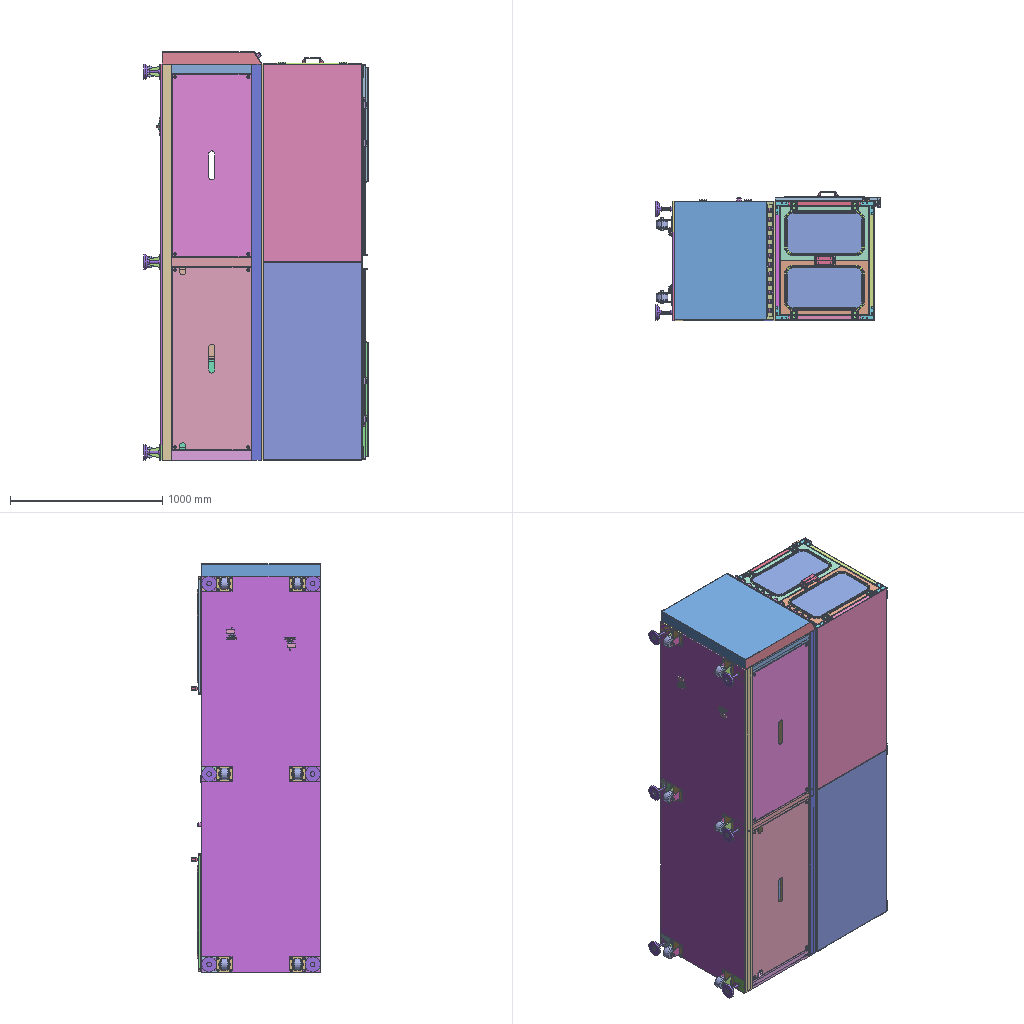Assembly | STEP file | 114 different items | 1060 placed | box 1475 x 845 x 2685 mm
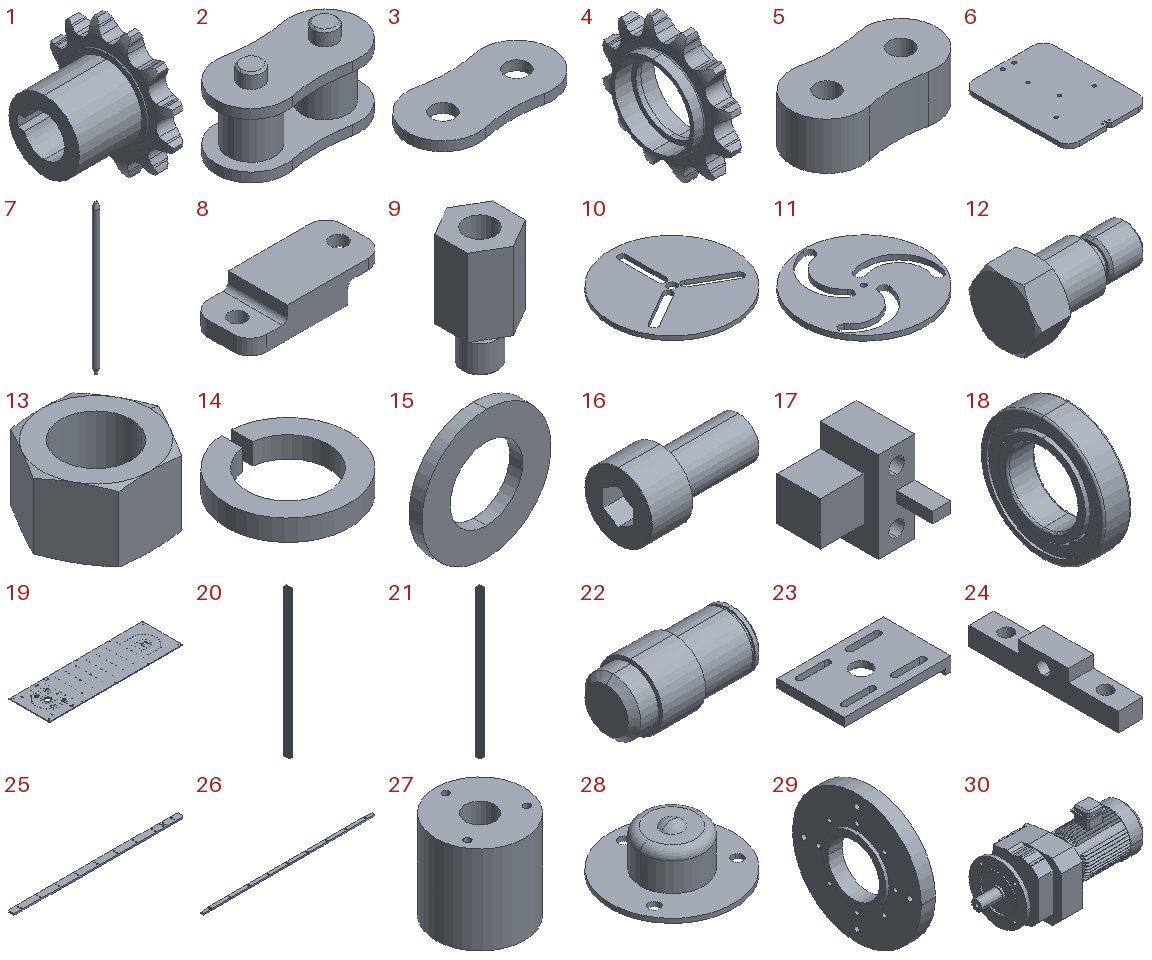Parts list (item | name | quantity | parent item | size | volume):
1 | Drive sprocket 16A-12_05B | x2 | in Chain assembly 16A (station pitch 254mm) | 70 x 105.245 x 105.245 mm | 183354 mm3
2 | Inner chain link | x80 | in Chain assembly 16A (station pitch 254mm) | 49.53 x 24.13 x 32 mm | 13899 mm3
3 | Outer chain link | x160 | in Chain assembly 16A (station pitch 254mm) | 49.79 x 24.39 x 3.25 mm | 3077 mm3
4 | Driven sprocket 16A-12_05B | x1 | in Chain assembly 16A (station pitch 254mm) | 32 x 105.245 x 105.245 mm | 65357 mm3
5 | Outer chain link pad block | x17 | in Chain assembly 16A (station pitch 254mm) | 49.79 x 24.39 x 16.175 mm | 15316 mm3
6 | Tray base | x16 | in Tooling | 180 x 235 x 10 mm | 413174 mm3
7 | Stop rod_default<machined> | x48 | in Tooling | 16 x 16 x 440 mm | 84922 mm3
8 | Guard rod seat | x48 | in Tooling | 80 x 35 x 18 mm | 32543 mm3
9 | M8X20 nut | x16 | in Tooling | 13 x 15.011 x 26.5 mm | 2477 mm3
10 | Tray plate-160 | x16 | in Tooling | 245 x 245 x 8 mm | 338994 mm3
11 | Rotary disc | x16 | in Tooling | 196 x 196 x 8 mm | 191240 mm3
12 | Tray bolt | x48 | in Tooling | 25.2 x 15.011 x 13 mm | 2145 mm3
13 | GB/T41-20001 type 1 hex nut, grade C, M8 | x48 | in Tooling | 14.2 x 12.298 x 7.9 mm | 635.641 mm3
14 | GB/T93-1987 standard spring lock washer (assembly) 8x2.1 | x48 | in Tooling | 12.277 x 12.254 x 2.1 mm | 135.755 mm3
15 | GB/T95-2002 plain washer grade C 8x1.6 | x48 | in Tooling | 16 x 1.6 x 16 mm | 219.911 mm3
16 | GB/T70.1-2000 socket head cap screw M8x16 | x16 | in Tooling | 24 x 13 x 13 mm | 1736 mm3
17 | Locating block | x16 | in Tooling | 22 x 26 x 25 mm | 4984 mm3
18 | GB/T276-94 deep groove ball bearing 6007-2Z | x2 | in Chain tooling assembly | 14 x 62 x 62 mm | 18417 mm3
19 | Silo large plate | x1 | in Silo assembly | 2600 x 780 x 12 mm | 23947596 mm3
20 | Industrial aluminium profile 3060 | x2 | in Silo assembly | 30 x 60 x 1500 mm | 776079 mm3
21 | Industrial aluminium profile 6060 | x1 | in Silo assembly | 60 x 60 x 1750 mm | 1492239 mm3
22 | Driven sprocket shaft | x1 | in Silo assembly | 79 x 40 x 40 mm | 82911 mm3
23 | Chain tension plate_default<machined> | x1 | in Silo assembly | 190 x 120 x 25 mm | 299042 mm3
24 | Driven sprocket expansion seat | x1 | in Silo assembly | 20 x 120 x 25 mm | 39515 mm3
25 | Nylon backrest plate 1 | x1 | in Silo assembly | 1900 x 69 x 16 mm | 2062797 mm3
26 | Outer nylon backrest plate 2 | x2 | in Silo assembly | 1500 x 30 x 12 mm | 516633 mm3
27 | Caster seat | x64 | in Silo assembly | 45 x 45 x 45 mm | 66141 mm3
28 | Caster wheel | x70 | in Silo assembly, Correction assembly | 45 x 45 x 17 mm | 7972 mm3
29 | Motor base plate | x1 | in Silo assembly | 27 x 200 x 200 mm | 543537 mm3
30 | NRFNRF57_NRF 27 | x1 | in Silo assembly | 502 x 221 x 222.6 mm | 8380262 mm3
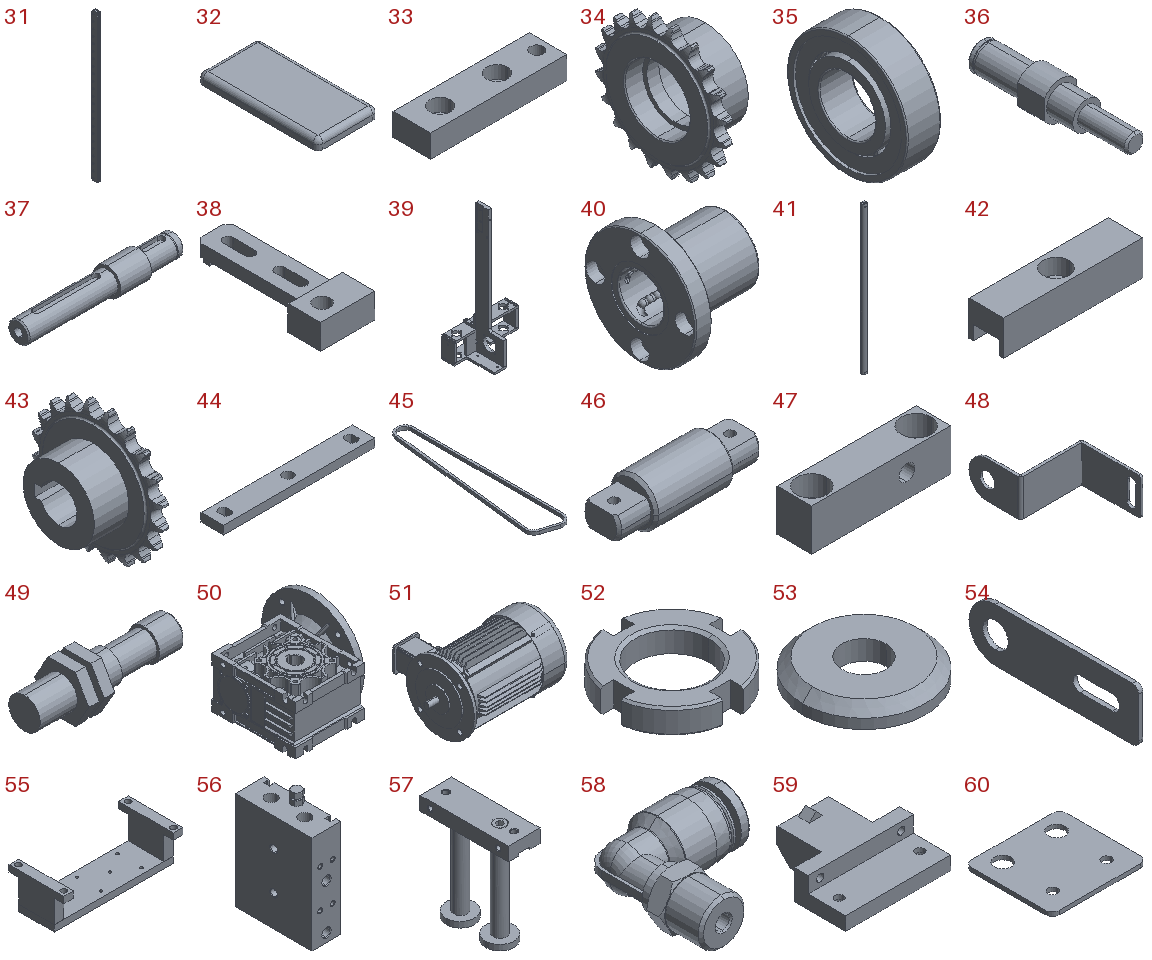31 | Flow rail_default<machined> | x4 | in Silo assembly | 46 x 62.5 x 1500 mm | 1123340 mm3
32 | Aluminium profile end cover plate | x4 | in Silo assembly | 30 x 60 x 5 mm | 8742 mm3
33 | Tensioning block | x10 | in Silo assembly | 72 x 20 x 12 mm | 15217 mm3
34 | Driven sprocket_05B | x4 | in Lifting mechanism | 24 x 64.324 x 64.324 mm | 22666 mm3
35 | Deep groove ball bearing 6002-2Z[GB/T276-94] | x8 | in Lifting mechanism | 9 x 32 x 32 mm | 3545 mm3
36 | Driven wheel shaft | x4 | in Lifting mechanism | 17 x 82.5 x 20 mm | 13654 mm3
37 | Reducer shaft | x2 | in Lifting mechanism | 131 x 23 x 23 mm | 35135 mm3
38 | Tensioner wheel bracket | x2 | in Lifting mechanism | 50 x 135 x 33 mm | 60411 mm3
39 | Lifting frame_default<machined> | x2 | in Lifting mechanism | 310 x 195 x 630 mm | 1240062 mm3
40 | LMFLMF20UU_LMF6UU | x8 | in Lifting mechanism | 42 x 54 x 54 mm | 26041 mm3
41 | Ejector rod | x4 | in Lifting mechanism | 20 x 20 x 620 mm | 192172 mm3
42 | Top plate part | x4 | in Lifting mechanism | 80 x 20 x 20 mm | 20619 mm3
43 | Drive sprocket_05B | x2 | in Lifting mechanism | 24 x 64.324 x 64.324 mm | 27131 mm3
44 | Link hanger plate | x2 | in Lifting mechanism | 270 x 40 x 15 mm | 150118 mm3
45 | Belt 1-2^Lifting mechanism | x2 | in Lifting mechanism | 133.82 x 674.32 x 12.8 mm | 154708 mm3
46 | Chain connecting rod | x2 | in Lifting mechanism | 54 x 18 x 18 mm | 10076 mm3
47 | Tensioning part | x2 | in Lifting mechanism | 60 x 15 x 18 mm | 12121 mm3
48 | Proximity switch bracket 2 | x2 | in Lifting mechanism | 52 x 90 x 30 mm | 7634 mm3
49 | Proximity switch | x6 | in Lifting mechanism, Positioning sensor assembly | 55.8 x 20.785 x 18 mm | 7139 mm3
50 | RV series aluminium alloy worm gear reducer RV40-63 | x2 | in Lifting mechanism | 120 x 160 x 140 mm | 864960 mm3
51 | Flanged end cover motor frame, no feet (TK) 63M | x2 | in Lifting mechanism | 231 x 187 x 140 mm | 1853530 mm3
52 | GB/T810-1988 small round nut M18x1.5 | x4 | in Lifting mechanism | 29.58 x 29.58 x 6 mm | 2282 mm3
53 | Small washer | x6 | in Lifting mechanism | 25 x 25 x 4 mm | 1560 mm3
54 | Proximity switch bracket 1 | x2 | in Lifting mechanism | 2 x 80 x 25 mm | 3345 mm3
55 | Cylinder mounting plate_default<machined> | x2 | in Correction assembly | 150 x 69 x 45 mm | 93928 mm3
56 | CXSM25-30(0_0)_BODY_HI | x2 | in CXSM25-30(0_0_0)_HI | 30 x 80 x 114 mm | 192548 mm3
57 | CXSM25-30(0_0)_ROD_HI | x2 | in CXSM25-30(0_0_0)_HI | 28 x 78 x 89 mm | 45235 mm3
58 | PL601_HI | x4 | in Correction assembly | 25.974 x 26.75 x 12.5 mm | 2654 mm3
59 | Correction clamp plate_default<machined> | x2 | in Correction assembly | 78 x 71 x 27 mm | 62305 mm3
60 | Sensor mounting plate | x1 | in Positioning sensor assembly | 70 x 65 x 3 mm | 12618 mm3
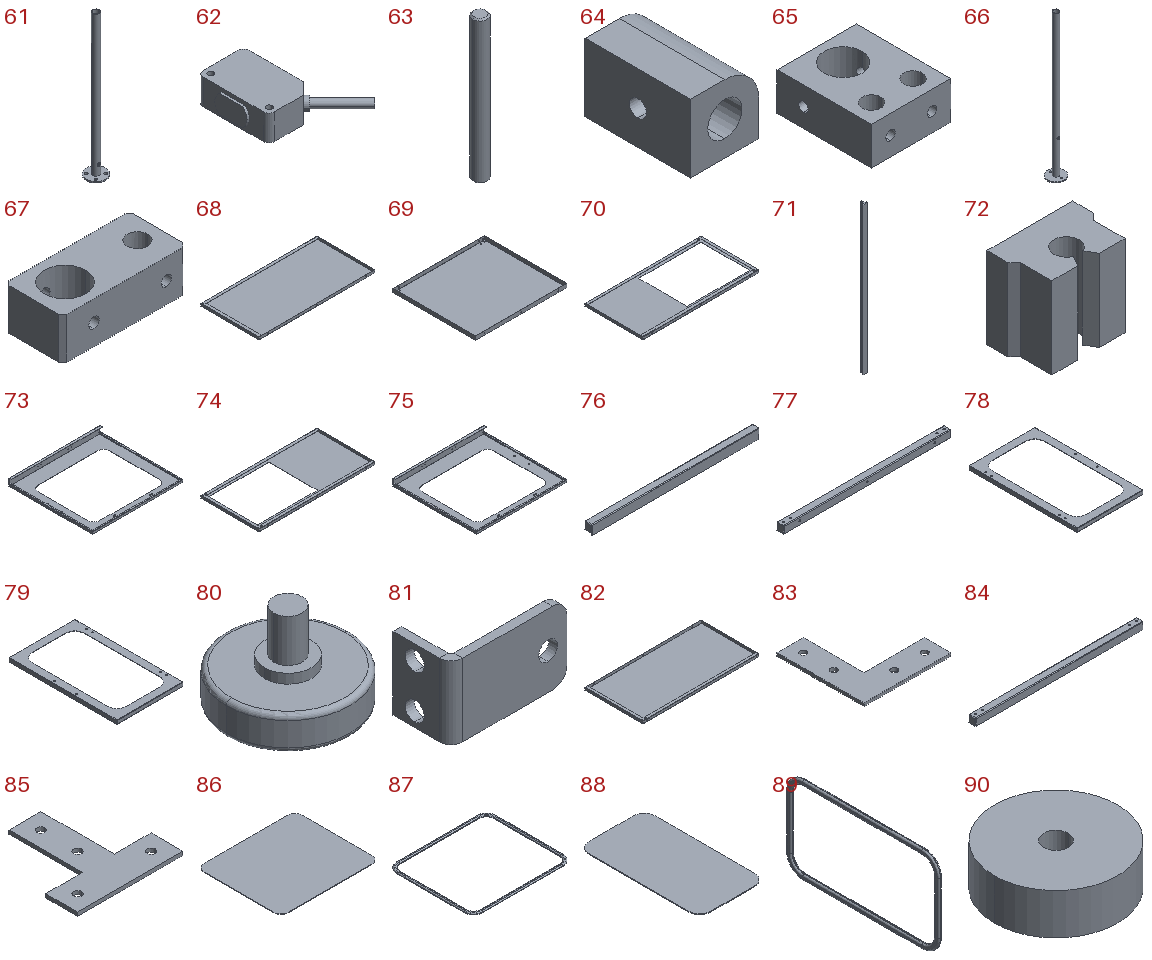61 | Switch support rod_default<machined> | x1 | in Detection mechanism | 60 x 60 x 440 mm | 47255 mm3
62 | Panasonic CX-444-P | x8 | in Detection mechanism, Sensor bracket, Sensor bracket 1 | 35.294 x 47.794 x 11.2 mm | 7023 mm3
63 | Small shaft | x8 | in Detection mechanism, Sensor bracket, Sensor bracket 1 | 10 x 10 x 100 mm | 7825 mm3
64 | Sensor mounting block | x8 | in Detection mechanism, Sensor bracket, Sensor bracket 1 | 20 x 31 x 20 mm | 9027 mm3
65 | Switch fixing block 2 | x2 | in Detection mechanism | 42 x 50 x 20 mm | 31937 mm3
66 | Switch support rod 1_default<machined> | x2 | in Sensor bracket, Sensor bracket 1 | 60 x 60 x 516 mm | 54480 mm3
67 | Switch fixing block 1 | x4 | in Sensor bracket, Sensor bracket 1 | 60 x 28 x 20 mm | 25066 mm3
68 | Inner sheet metal 1 | x1 | in Sheet metal guard | 1300 x 650 x 30 mm | 1507890 mm3
69 | Rear sheet metal | x1 | in Sheet metal guard | 720 x 650 x 30 mm | 814414 mm3
70 | Outer sheet metal | x1 | in Sheet metal guard | 1300 x 650 x 30 mm | 960013 mm3
71 | SBR16S round rail_default<machined> | x2 | in Sheet metal guard | 30 x 28.5 x 1020 mm | 387317 mm3
72 | SBR16S slide rail | x4 | in Sheet metal guard | 41 x 28 x 39 mm | 34697 mm3
73 | Sheet metal sliding door 1 | x1 | in Sheet metal guard | 750 x 690 x 61 mm | 498963 mm3
74 | Outer sheet metal 1 | x1 | in Sheet metal guard | 1300 x 650 x 30 mm | 959782 mm3
75 | Sheet metal sliding door | x1 | in Sheet metal guard | 750 x 690 x 61 mm | 498963 mm3
76 | Front sheet metal baffle | x1 | in Sheet metal guard | 720 x 30 x 40 mm | 104570 mm3
77 | Front lower sheet metal baffle | x1 | in Sheet metal guard | 720 x 30 x 30 mm | 93839 mm3
78 | Sheet metal front door | x1 | in Sheet metal guard | 360 x 588 x 21.5 mm | 195995 mm3
79 | Sheet metal front door 1 | x1 | in Sheet metal guard | 360 x 588 x 21.5 mm | 195995 mm3
80 | Nylon roller | x4 | in Sheet metal guard | 26 x 26 x 18 mm | 4094 mm3
81 | Roller hanger plate | x4 | in Sheet metal guard | 40 x 20 x 25 mm | 3864 mm3
82 | Inner sheet metal | x1 | in Sheet metal guard | 1300 x 650 x 30 mm | 1507394 mm3
83 | Outer connecting plate | x12 | in Sheet metal guard | 86 x 86 x 3 mm | 10990 mm3
84 | Middle sheet metal support plate | x1 | in Sheet metal guard | 720 x 30 x 30 mm | 93836 mm3
85 | Outer connecting plate L | x2 | in Sheet metal guard | 86 x 86 x 3 mm | 10990 mm3
86 | Glass plate | x2 | in Sheet metal guard | 580 x 500 x 3 mm | 864785 mm3
87 | Part 6^Sheet metal guard | x2 | in Sheet metal guard | 607.906 x 527.906 x 12 mm | 319171 mm3
88 | Glass plate 1 | x2 | in Sheet metal guard | 270 x 498 x 3 mm | 398165 mm3
89 | Part 8^Sheet metal guard | x2 | in Sheet metal guard | 12 x 525.906 x 297.906 mm | 225066 mm3
90 | Small locating block | x4 | in Sheet metal guard | 30 x 30 x 10 mm | 6786 mm3
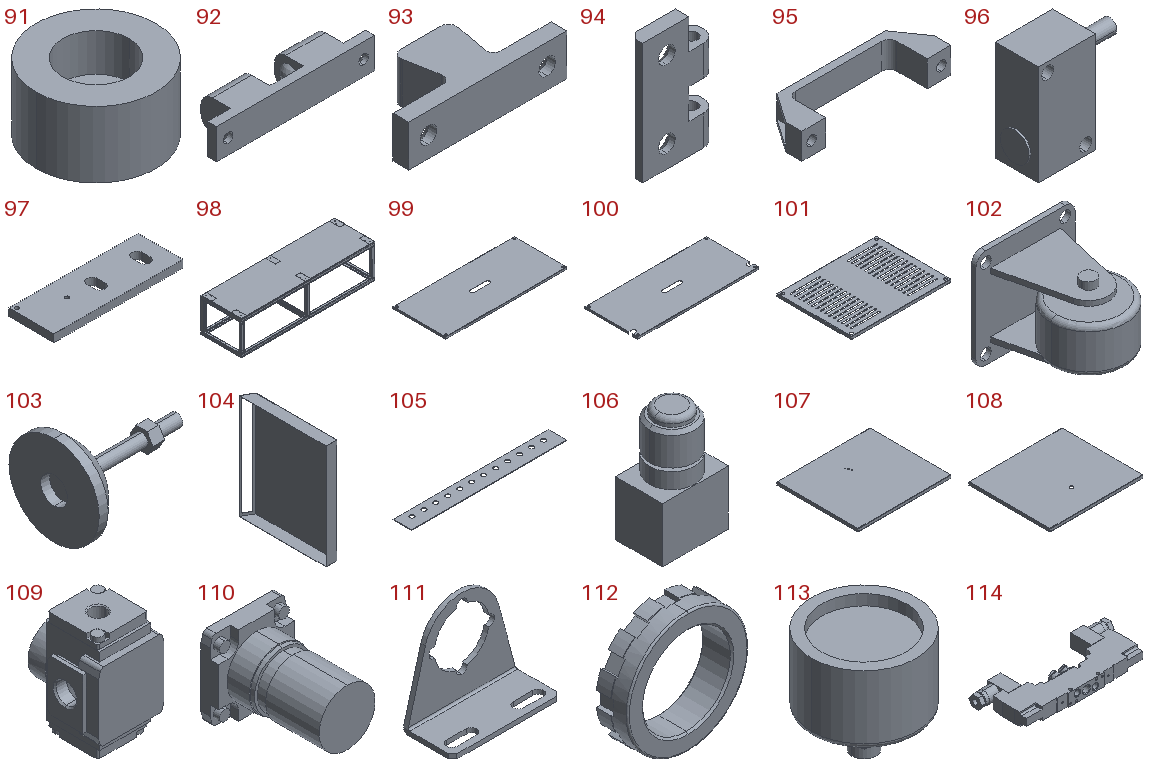91 | Buffer block | x2 | in Sheet metal guard | 18 x 18 x 10 mm | 2002 mm3
92 | Ball catch 1 | x6 | in Sheet metal guard, Box assembly | 70 x 17 x 13.5 mm | 9503 mm3
93 | Ball catch 2 | x6 | in Sheet metal guard, Box assembly | 40 x 17 x 10.5 mm | 3213 mm3
94 | Hinge CE-H3030-8-ZN | x16 | in Sheet metal guard, Box assembly | 29.8 x 10 x 49.2 mm | 6093 mm3
95 | Handle 180 | x4 | in Sheet metal guard | 138 x 42 x 24 mm | 35568 mm3
96 | Square proximity switch | x4 | in Sheet metal guard | 26.5 x 12 x 28 mm | 5309 mm3
97 | Square proximity switch plate | x2 | in Sheet metal guard | 86 x 30 x 5 mm | 12116 mm3
98 | Box 1_default<machined> | x1 | in Box assembly | 2600 x 780 x 662 mm | 45698712 mm3
99 | Box sheet metal 1_default<machined> | x2 | in Box assembly | 1203 x 522 x 20 mm | 1037743 mm3
100 | Box sheet metal 2_default<machined> | x1 | in Box assembly | 1203 x 522 x 20 mm | 1030115 mm3
101 | Box sheet metal_default<machined> | x1 | in Box assembly | 698 x 522 x 20 mm | 532626 mm3
102 | Caster_default<machined> | x6 | in Box assembly | 100 x 106 x 100 mm | 289989 mm3
103 | Foot | x6 | in Box assembly | 136 x 100 x 100 mm | 184245 mm3
104 | Push button box_default<machined> | x1 | in Box assembly | 80 x 650.121 x 780 mm | 985013 mm3
105 | Push button cover plate | x1 | in Box assembly | 780 x 92 x 3 mm | 201595 mm3
106 | Push button | x13 | in Box assembly | 42 x 30 x 72 mm | 66277 mm3
107 | Box door_default<machined> | x1 | in Box assembly | 600 x 522 x 20 mm | 571092 mm3
108 | Box door 1_default<machined> | x1 | in Box assembly | 600 x 522 x 20 mm | 570664 mm3
109 | AR20-02G(0)_BODY_HI | x1 | in AR20-02BG(0)_HI | 40 x 42.9 x 57 mm | 61556 mm3
110 | AR-20_BONNET_HI | x1 | in AR20-02BG(0)_HI | 36 x 51.1 x 37.5 mm | 33945 mm3
111 | AR20P-270AS(20)_BRACKET_HI | x1 | in AR20-02BG(0)_HI | 55 x 25.2 x 49.3 mm | 5580 mm3
112 | AR20P-260S(20)_SETNUT_HI | x1 | in AR20-02BG(0)_HI | 37.229 x 9.5 x 37.229 mm | 4541 mm3
113 | AR20-G_GAUGE_HI | x1 | in AR20-02BG(0)_HI | 37.5 x 37.5 x 37.5 mm | 25733 mm3
114 | VQZ2220-5YZ1-C6_V2_HI | x1 | in VQZ2220-5YZ1-C6_HI | 159.8 x 61.406 x 15.8 mm | 81449 mm3
Placements (level | parent | child | x y z in mm | rotation matrix by rows), first 278 of 1093 lines:
1 | subassembly 2 | Chain tooling assembly | -233.53 14.629 0.1141 | 1 0 0 0 1 0 0 0 1
2 | Chain tooling assembly | Chain assembly 16A (station pitch 254mm) | 38.756 -73.811 -756.814 | 1 0 0 0 1 0 0 0 1
3 | Chain assembly 16A (station pitch 254mm) | Drive sprocket 16A-12_05B | -13.434 74.292 1696.51 | 1 0 0 0 0.9659 -0.2588 0 0.2588 0.9659
3 | Chain assembly 16A (station pitch 254mm) | Inner chain link | -13.486 33.245 1720.208 | 0 0 -1 -0.5 -0.866 0 -0.866 0.5 0
3 | Chain assembly 16A (station pitch 254mm) | Inner chain link | -13.486 74.292 1743.907 | 0 0 -1 -1 0 0 0 1 0
3 | Chain assembly 16A (station pitch 254mm) | Inner chain link | -13.486 115.339 1720.208 | 0 0 -1 0.5 -0.866 0 -0.866 -0.5 -0
3 | Chain assembly 16A (station pitch 254mm) | Outer chain link | 0.8895 26.895 1696.51 | 0 0 -1 0 1 0 1 0 0
3 | Chain assembly 16A (station pitch 254mm) | Outer chain link | 0.8895 97.99 1737.557 | 0 0 -1 -0.866 0.5 0 0.5 0.866 0
3 | Chain assembly 16A (station pitch 254mm) | Outer chain link | 0.8895 50.593 1737.557 | 0 0 -1 -0.866 -0.5 0 -0.5 0.866 0
3 | Chain assembly 16A (station pitch 254mm) | Inner chain link | -13.486 121.689 1671.11 | 0 0 -1 0 -1 0 -1 0 -0
3 | Chain assembly 16A (station pitch 254mm) | Outer chain link | 0.8895 121.689 1696.51 | 0 0 -1 0 1 0 1 0 -0
3 | Chain assembly 16A (station pitch 254mm) | Inner chain link | -13.486 26.895 1671.11 | 0 0 -1 0 -1 0 -1 0 -0
3 | Chain assembly 16A (station pitch 254mm) | Outer chain link | 0.8895 121.689 1645.71 | 0 0 -1 0 1 0 1 0 -0
3 | Chain assembly 16A (station pitch 254mm) | Outer chain link | -24.61 121.689 1645.71 | 0 0 -1 0 1 0 1 0 -0
3 | Chain assembly 16A (station pitch 254mm) | Inner chain link | -13.486 121.689 1620.31 | 0 0 -1 0 -1 0 -1 0 -0
3 | Chain assembly 16A (station pitch 254mm) | Outer chain link | 0.8895 26.895 1645.71 | 0 0 -1 0 1 0 1 0 -0
3 | Chain assembly 16A (station pitch 254mm) | Outer chain link | -24.61 26.895 1645.71 | 0 0 -1 0 1 0 1 0 -0
3 | Chain assembly 16A (station pitch 254mm) | Inner chain link | -13.486 26.895 1620.31 | 0 0 -1 0 -1 0 -1 0 -0
3 | Chain assembly 16A (station pitch 254mm) | Outer chain link | -24.61 121.686 1594.91 | 0 0 -1 0 1 0 1 0 -0
3 | Chain assembly 16A (station pitch 254mm) | Outer chain link | -24.61 121.684 1544.11 | 0 0 -1 0 1 0 1 0 -0
3 | Chain assembly 16A (station pitch 254mm) | Outer chain link | -24.61 121.682 1493.31 | 0 0 -1 0 1 0 1 0 -0
3 | Chain assembly 16A (station pitch 254mm) | Outer chain link | -24.61 121.68 1442.51 | 0 0 -1 0 1 0 1 0 -0
3 | Chain assembly 16A (station pitch 254mm) | Outer chain link | -24.61 121.677 1391.71 | 0 0 -1 0 1 0 1 0 -0
3 | Chain assembly 16A (station pitch 254mm) | Outer chain link | -24.61 121.675 1340.91 | 0 0 -1 0 1 0 1 0 -0
3 | Chain assembly 16A (station pitch 254mm) | Outer chain link | -24.61 121.673 1290.11 | 0 0 -1 0 1 0 1 0 -0
3 | Chain assembly 16A (station pitch 254mm) | Outer chain link | -24.61 121.671 1239.31 | 0 0 -1 0 1 0 1 0 -0
3 | Chain assembly 16A (station pitch 254mm) | Outer chain link | -24.61 121.668 1188.51 | 0 0 -1 0 1 0 1 0 -0
3 | Chain assembly 16A (station pitch 254mm) | Outer chain link | -24.61 121.666 1137.71 | 0 0 -1 0 1 0 1 0 -0
3 | Chain assembly 16A (station pitch 254mm) | Outer chain link | -24.61 121.664 1086.91 | 0 0 -1 0 1 0 1 0 -0
3 | Chain assembly 16A (station pitch 254mm) | Outer chain link | -24.61 121.662 1036.11 | 0 0 -1 0 1 0 1 0 -0
3 | Chain assembly 16A (station pitch 254mm) | Outer chain link | -24.61 121.659 985.31 | 0 0 -1 0 1 0 1 0 -0
3 | Chain assembly 16A (station pitch 254mm) | Outer chain link | -24.61 121.657 934.51 | 0 0 -1 0 1 0 1 0 -0
3 | Chain assembly 16A (station pitch 254mm) | Outer chain link | -24.61 121.655 883.71 | 0 0 -1 0 1 0 1 0 -0
3 | Chain assembly 16A (station pitch 254mm) | Outer chain link | -24.61 121.653 832.91 | 0 0 -1 0 1 0 1 0 -0
3 | Chain assembly 16A (station pitch 254mm) | Outer chain link | -24.61 121.65 782.11 | 0 0 -1 0 1 0 1 0 -0
3 | Chain assembly 16A (station pitch 254mm) | Outer chain link | -24.61 121.648 731.31 | 0 0 -1 0 1 0 1 0 -0
3 | Chain assembly 16A (station pitch 254mm) | Outer chain link | -24.61 121.646 680.51 | 0 0 -1 0 1 0 1 0 -0
3 | Chain assembly 16A (station pitch 254mm) | Outer chain link | -24.61 121.644 629.71 | 0 0 -1 0 1 0 1 0 -0
3 | Chain assembly 16A (station pitch 254mm) | Outer chain link | -24.61 121.641 578.91 | 0 0 -1 0 1 0 1 0 -0
3 | Chain assembly 16A (station pitch 254mm) | Outer chain link | -24.61 121.639 528.11 | 0 0 -1 0 1 0 1 0 -0
3 | Chain assembly 16A (station pitch 254mm) | Outer chain link | -24.61 121.637 477.31 | 0 0 -1 0 1 0 1 0 -0
3 | Chain assembly 16A (station pitch 254mm) | Outer chain link | -24.61 121.634 426.51 | 0 0 -1 0 1 0 1 0 -0
3 | Chain assembly 16A (station pitch 254mm) | Outer chain link | -24.61 121.632 375.71 | 0 0 -1 0 1 0 1 0 -0
3 | Chain assembly 16A (station pitch 254mm) | Outer chain link | -24.61 121.63 324.91 | 0 0 -1 0 1 0 1 0 -0
3 | Chain assembly 16A (station pitch 254mm) | Outer chain link | -24.61 121.628 274.11 | 0 0 -1 0 1 0 1 0 -0
3 | Chain assembly 16A (station pitch 254mm) | Outer chain link | -24.61 121.625 223.31 | 0 0 -1 0 1 0 1 0 -0
3 | Chain assembly 16A (station pitch 254mm) | Outer chain link | -24.61 121.623 172.51 | 0 0 -1 0 1 0 1 0 -0
3 | Chain assembly 16A (station pitch 254mm) | Outer chain link | -24.61 121.621 121.71 | 0 0 -1 0 1 0 1 0 -0
3 | Chain assembly 16A (station pitch 254mm) | Outer chain link | -24.61 121.619 70.91 | 0 0 -1 0 1 0 1 0 -0
3 | Chain assembly 16A (station pitch 254mm) | Outer chain link | -24.61 121.616 20.11 | 0 0 -1 0 1 0 1 0 -0
3 | Chain assembly 16A (station pitch 254mm) | Outer chain link | -24.61 121.614 -30.69 | 0 0 -1 0 1 0 1 0 -0
3 | Chain assembly 16A (station pitch 254mm) | Outer chain link | -24.61 121.612 -81.49 | 0 0 -1 0 1 0 1 0 -0
3 | Chain assembly 16A (station pitch 254mm) | Outer chain link | -24.61 121.609 -132.29 | 0 0 -1 0 1 0 1 0 -0
3 | Chain assembly 16A (station pitch 254mm) | Outer chain link | 0.8895 121.686 1594.91 | 0 0 -1 0 1 0 1 0 -0
3 | Chain assembly 16A (station pitch 254mm) | Outer chain link | 0.8895 121.684 1544.11 | 0 0 -1 0 1 0 1 0 -0
3 | Chain assembly 16A (station pitch 254mm) | Outer chain link | 0.8895 121.682 1493.31 | 0 0 -1 0 1 0 1 0 -0
3 | Chain assembly 16A (station pitch 254mm) | Outer chain link | 0.8895 121.68 1442.51 | 0 0 -1 0 1 0 1 0 -0
3 | Chain assembly 16A (station pitch 254mm) | Outer chain link | 0.8895 121.677 1391.71 | 0 0 -1 0 1 0 1 0 -0
3 | Chain assembly 16A (station pitch 254mm) | Outer chain link | 0.8895 121.675 1340.91 | 0 0 -1 0 1 0 1 0 -0
3 | Chain assembly 16A (station pitch 254mm) | Outer chain link | 0.8895 121.673 1290.11 | 0 0 -1 0 1 0 1 0 -0
3 | Chain assembly 16A (station pitch 254mm) | Outer chain link | 0.8895 121.671 1239.31 | 0 0 -1 0 1 0 1 0 -0
3 | Chain assembly 16A (station pitch 254mm) | Outer chain link | 0.8895 121.668 1188.51 | 0 0 -1 0 1 0 1 0 -0
3 | Chain assembly 16A (station pitch 254mm) | Outer chain link | 0.8895 121.666 1137.71 | 0 0 -1 0 1 0 1 0 -0
3 | Chain assembly 16A (station pitch 254mm) | Outer chain link | 0.8895 121.664 1086.91 | 0 0 -1 0 1 0 1 0 -0
3 | Chain assembly 16A (station pitch 254mm) | Outer chain link | 0.8895 121.662 1036.11 | 0 0 -1 0 1 0 1 0 -0
3 | Chain assembly 16A (station pitch 254mm) | Outer chain link | 0.8895 121.659 985.31 | 0 0 -1 0 1 0 1 0 -0
3 | Chain assembly 16A (station pitch 254mm) | Outer chain link | 0.8895 121.657 934.51 | 0 0 -1 0 1 0 1 0 -0
3 | Chain assembly 16A (station pitch 254mm) | Outer chain link | 0.8895 121.655 883.71 | 0 0 -1 0 1 0 1 0 -0
3 | Chain assembly 16A (station pitch 254mm) | Outer chain link | 0.8895 121.653 832.91 | 0 0 -1 0 1 0 1 0 -0
3 | Chain assembly 16A (station pitch 254mm) | Outer chain link | 0.8895 121.65 782.11 | 0 0 -1 0 1 0 1 0 -0
3 | Chain assembly 16A (station pitch 254mm) | Outer chain link | 0.8895 121.648 731.31 | 0 0 -1 0 1 0 1 0 -0
3 | Chain assembly 16A (station pitch 254mm) | Outer chain link | 0.8895 121.646 680.51 | 0 0 -1 0 1 0 1 0 -0
3 | Chain assembly 16A (station pitch 254mm) | Outer chain link | 0.8895 121.644 629.71 | 0 0 -1 0 1 0 1 0 -0
3 | Chain assembly 16A (station pitch 254mm) | Outer chain link | 0.8895 121.641 578.91 | 0 0 -1 0 1 0 1 0 -0
3 | Chain assembly 16A (station pitch 254mm) | Outer chain link | 0.8895 121.639 528.11 | 0 0 -1 0 1 0 1 0 -0
3 | Chain assembly 16A (station pitch 254mm) | Outer chain link | 0.8895 121.637 477.31 | 0 0 -1 0 1 0 1 0 -0
3 | Chain assembly 16A (station pitch 254mm) | Outer chain link | 0.8895 121.634 426.51 | 0 0 -1 0 1 0 1 0 -0
3 | Chain assembly 16A (station pitch 254mm) | Outer chain link | 0.8895 121.632 375.71 | 0 0 -1 0 1 0 1 0 -0
3 | Chain assembly 16A (station pitch 254mm) | Outer chain link | 0.8895 121.63 324.91 | 0 0 -1 0 1 0 1 0 -0
3 | Chain assembly 16A (station pitch 254mm) | Outer chain link | 0.8895 121.628 274.11 | 0 0 -1 0 1 0 1 0 -0
3 | Chain assembly 16A (station pitch 254mm) | Outer chain link | 0.8895 121.625 223.31 | 0 0 -1 0 1 0 1 0 -0
3 | Chain assembly 16A (station pitch 254mm) | Outer chain link | 0.8895 121.623 172.51 | 0 0 -1 0 1 0 1 0 -0
3 | Chain assembly 16A (station pitch 254mm) | Outer chain link | 0.8895 121.621 121.71 | 0 0 -1 0 1 0 1 0 -0
3 | Chain assembly 16A (station pitch 254mm) | Outer chain link | 0.8895 121.619 70.91 | 0 0 -1 0 1 0 1 0 -0
3 | Chain assembly 16A (station pitch 254mm) | Outer chain link | 0.8895 121.616 20.11 | 0 0 -1 0 1 0 1 0 -0
3 | Chain assembly 16A (station pitch 254mm) | Outer chain link | 0.8895 121.614 -30.69 | 0 0 -1 0 1 0 1 0 -0
3 | Chain assembly 16A (station pitch 254mm) | Outer chain link | 0.8895 121.612 -81.49 | 0 0 -1 0 1 0 1 0 -0
3 | Chain assembly 16A (station pitch 254mm) | Outer chain link | 1.25 121.609 -132.29 | 0 0 -1 0 1 0 1 0 -0
3 | Chain assembly 16A (station pitch 254mm) | Inner chain link | -13.486 121.686 1569.51 | 0 0 -1 0 -1 0 -1 0 -0
3 | Chain assembly 16A (station pitch 254mm) | Inner chain link | -13.486 121.684 1518.71 | 0 0 -1 0 -1 0 -1 0 -0
3 | Chain assembly 16A (station pitch 254mm) | Inner chain link | -13.486 121.682 1467.91 | 0 0 -1 0 -1 0 -1 0 -0
3 | Chain assembly 16A (station pitch 254mm) | Inner chain link | -13.486 121.68 1417.11 | 0 0 -1 0 -1 0 -1 0 -0
3 | Chain assembly 16A (station pitch 254mm) | Inner chain link | -13.486 121.677 1366.31 | 0 0 -1 0 -1 0 -1 0 -0
3 | Chain assembly 16A (station pitch 254mm) | Inner chain link | -13.486 121.675 1315.51 | 0 0 -1 0 -1 0 -1 0 -0
3 | Chain assembly 16A (station pitch 254mm) | Inner chain link | -13.486 121.673 1264.71 | 0 0 -1 0 -1 0 -1 0 -0
3 | Chain assembly 16A (station pitch 254mm) | Inner chain link | -13.486 121.671 1213.91 | 0 0 -1 0 -1 0 -1 0 -0
3 | Chain assembly 16A (station pitch 254mm) | Inner chain link | -13.486 121.668 1163.11 | 0 0 -1 0 -1 0 -1 0 -0
3 | Chain assembly 16A (station pitch 254mm) | Inner chain link | -13.486 121.666 1112.31 | 0 0 -1 0 -1 0 -1 0 -0
3 | Chain assembly 16A (station pitch 254mm) | Inner chain link | -13.486 121.664 1061.51 | 0 0 -1 0 -1 0 -1 0 -0
3 | Chain assembly 16A (station pitch 254mm) | Inner chain link | -13.486 121.662 1010.71 | 0 0 -1 0 -1 0 -1 0 -0
3 | Chain assembly 16A (station pitch 254mm) | Inner chain link | -13.486 121.659 959.91 | 0 0 -1 0 -1 0 -1 0 -0
3 | Chain assembly 16A (station pitch 254mm) | Inner chain link | -13.486 121.657 909.11 | 0 0 -1 0 -1 0 -1 0 -0
3 | Chain assembly 16A (station pitch 254mm) | Inner chain link | -13.486 121.655 858.31 | 0 0 -1 0 -1 0 -1 0 -0
3 | Chain assembly 16A (station pitch 254mm) | Inner chain link | -13.486 121.653 807.51 | 0 0 -1 0 -1 0 -1 0 -0
3 | Chain assembly 16A (station pitch 254mm) | Inner chain link | -13.486 121.65 756.71 | 0 0 -1 0 -1 0 -1 0 -0
3 | Chain assembly 16A (station pitch 254mm) | Inner chain link | -13.486 121.648 705.91 | 0 0 -1 0 -1 0 -1 0 -0
3 | Chain assembly 16A (station pitch 254mm) | Inner chain link | -13.486 121.646 655.11 | 0 0 -1 0 -1 0 -1 0 -0
3 | Chain assembly 16A (station pitch 254mm) | Inner chain link | -13.486 121.644 604.31 | 0 0 -1 0 -1 0 -1 0 -0
3 | Chain assembly 16A (station pitch 254mm) | Inner chain link | -13.486 121.641 553.51 | 0 0 -1 0 -1 0 -1 0 -0
3 | Chain assembly 16A (station pitch 254mm) | Inner chain link | -13.486 121.639 502.71 | 0 0 -1 0 -1 0 -1 0 -0
3 | Chain assembly 16A (station pitch 254mm) | Inner chain link | -13.486 121.637 451.91 | 0 0 -1 0 -1 0 -1 0 -0
3 | Chain assembly 16A (station pitch 254mm) | Inner chain link | -13.486 121.634 401.11 | 0 0 -1 0 -1 0 -1 0 -0
3 | Chain assembly 16A (station pitch 254mm) | Inner chain link | -13.486 121.632 350.31 | 0 0 -1 0 -1 0 -1 0 -0
3 | Chain assembly 16A (station pitch 254mm) | Inner chain link | -13.486 121.63 299.51 | 0 0 -1 0 -1 0 -1 0 -0
3 | Chain assembly 16A (station pitch 254mm) | Inner chain link | -13.486 121.628 248.71 | 0 0 -1 0 -1 0 -1 0 -0
3 | Chain assembly 16A (station pitch 254mm) | Inner chain link | -13.486 121.625 197.91 | 0 0 -1 0 -1 0 -1 0 -0
3 | Chain assembly 16A (station pitch 254mm) | Inner chain link | -13.486 121.623 147.11 | 0 0 -1 0 -1 0 -1 0 -0
3 | Chain assembly 16A (station pitch 254mm) | Inner chain link | -13.486 121.621 96.31 | 0 0 -1 0 -1 0 -1 0 -0
3 | Chain assembly 16A (station pitch 254mm) | Inner chain link | -13.486 121.619 45.51 | 0 0 -1 0 -1 0 -1 0 -0
3 | Chain assembly 16A (station pitch 254mm) | Inner chain link | -13.486 121.616 -5.29 | 0 0 -1 0 -1 0 -1 0 -0
3 | Chain assembly 16A (station pitch 254mm) | Inner chain link | -13.486 121.614 -56.09 | 0 0 -1 0 -1 0 -1 0 -0
3 | Chain assembly 16A (station pitch 254mm) | Inner chain link | -13.486 121.612 -106.891 | 0 0 -1 0 -1 0 -1 0 -0
3 | Chain assembly 16A (station pitch 254mm) | Inner chain link | -13.486 121.609 -157.69 | 0 0 -1 0 -1 0 -1 0 -0
3 | Chain assembly 16A (station pitch 254mm) | Driven sprocket 16A-12_05B | -13.434 74.292 -183.09 | 1 0 0 0 0.9659 -0.2588 0 0.2588 0.9659
3 | Chain assembly 16A (station pitch 254mm) | Outer chain link | 0.8895 26.895 1594.91 | 0 0 -1 0 1 0 1 0 -0
3 | Chain assembly 16A (station pitch 254mm) | Outer chain link | 0.8895 26.895 1544.11 | 0 0 -1 0 1 0 1 0 -0
3 | Chain assembly 16A (station pitch 254mm) | Outer chain link | 0.8895 26.895 1493.31 | 0 0 -1 0 1 0 1 0 -0
3 | Chain assembly 16A (station pitch 254mm) | Outer chain link | 0.8895 26.895 1442.51 | 0 0 -1 0 1 0 1 0 -0
3 | Chain assembly 16A (station pitch 254mm) | Outer chain link | 0.8895 26.895 1391.71 | 0 0 -1 0 1 0 1 0 -0
3 | Chain assembly 16A (station pitch 254mm) | Outer chain link | 0.8895 26.895 1340.91 | 0 0 -1 0 1 0 1 0 -0
3 | Chain assembly 16A (station pitch 254mm) | Outer chain link | 0.8895 26.895 1290.11 | 0 0 -1 0 1 0 1 0 -0
3 | Chain assembly 16A (station pitch 254mm) | Outer chain link | 0.8895 26.895 1239.31 | 0 0 -1 0 1 0 1 0 -0
3 | Chain assembly 16A (station pitch 254mm) | Outer chain link | 0.8895 26.895 1188.51 | 0 0 -1 0 1 0 1 0 -0
3 | Chain assembly 16A (station pitch 254mm) | Outer chain link | 0.8895 26.895 1137.71 | 0 0 -1 0 1 0 1 0 -0
3 | Chain assembly 16A (station pitch 254mm) | Outer chain link | 0.8895 26.895 1086.91 | 0 0 -1 0 1 0 1 0 -0
3 | Chain assembly 16A (station pitch 254mm) | Outer chain link | 0.8895 26.895 1036.11 | 0 0 -1 0 1 0 1 0 -0
3 | Chain assembly 16A (station pitch 254mm) | Outer chain link | 0.8895 26.895 985.31 | 0 0 -1 0 1 0 1 0 -0
3 | Chain assembly 16A (station pitch 254mm) | Outer chain link | 0.8895 26.895 934.51 | 0 0 -1 0 1 0 1 0 -0
3 | Chain assembly 16A (station pitch 254mm) | Outer chain link | 0.8895 26.895 883.71 | 0 0 -1 0 1 0 1 0 -0
3 | Chain assembly 16A (station pitch 254mm) | Outer chain link | 0.8895 26.895 832.91 | 0 0 -1 0 1 0 1 0 -0
3 | Chain assembly 16A (station pitch 254mm) | Outer chain link | 0.8895 26.895 782.11 | 0 0 -1 0 1 0 1 0 -0
3 | Chain assembly 16A (station pitch 254mm) | Outer chain link | 0.8895 26.895 731.31 | 0 0 -1 0 1 0 1 0 -0
3 | Chain assembly 16A (station pitch 254mm) | Outer chain link | 0.8895 26.895 680.51 | 0 0 -1 0 1 0 1 0 -0
3 | Chain assembly 16A (station pitch 254mm) | Outer chain link | 0.8895 26.895 629.71 | 0 0 -1 0 1 0 1 0 -0
3 | Chain assembly 16A (station pitch 254mm) | Outer chain link | 0.8895 26.895 578.91 | 0 0 -1 0 1 0 1 0 -0
3 | Chain assembly 16A (station pitch 254mm) | Outer chain link | 0.8895 26.895 528.11 | 0 0 -1 0 1 0 1 0 -0
3 | Chain assembly 16A (station pitch 254mm) | Outer chain link | 0.8895 26.895 477.31 | 0 0 -1 0 1 0 1 0 -0
3 | Chain assembly 16A (station pitch 254mm) | Outer chain link | 0.8895 26.895 426.51 | 0 0 -1 0 1 0 1 0 -0
3 | Chain assembly 16A (station pitch 254mm) | Outer chain link | 0.8895 26.895 375.71 | 0 0 -1 0 1 0 1 0 -0
3 | Chain assembly 16A (station pitch 254mm) | Outer chain link | 0.8895 26.895 324.91 | 0 0 -1 0 1 0 1 0 -0
3 | Chain assembly 16A (station pitch 254mm) | Outer chain link | 0.8895 26.895 274.11 | 0 0 -1 0 1 0 1 0 -0
3 | Chain assembly 16A (station pitch 254mm) | Outer chain link | 0.8895 26.895 223.31 | 0 0 -1 0 1 0 1 0 -0
3 | Chain assembly 16A (station pitch 254mm) | Outer chain link | 0.8895 26.895 172.51 | 0 0 -1 0 1 0 1 0 -0
3 | Chain assembly 16A (station pitch 254mm) | Outer chain link | 0.8895 26.895 121.71 | 0 0 -1 0 1 0 1 0 -0
3 | Chain assembly 16A (station pitch 254mm) | Outer chain link | 0.8895 26.895 70.91 | 0 0 -1 0 1 0 1 0 -0
3 | Chain assembly 16A (station pitch 254mm) | Outer chain link | 0.8895 26.895 20.11 | 0 0 -1 0 1 0 1 0 -0
3 | Chain assembly 16A (station pitch 254mm) | Outer chain link | 0.8895 26.895 -30.69 | 0 0 -1 0 1 0 1 0 -0
3 | Chain assembly 16A (station pitch 254mm) | Outer chain link | 0.8895 26.895 -81.49 | 0 0 -1 0 1 0 1 0 -0
3 | Chain assembly 16A (station pitch 254mm) | Outer chain link | 1.25 26.895 -132.29 | 0 0 -1 0 1 0 1 0 -0
3 | Chain assembly 16A (station pitch 254mm) | Outer chain link | -24.61 26.895 1594.91 | 0 0 -1 0 1 0 1 0 -0
3 | Chain assembly 16A (station pitch 254mm) | Outer chain link | -24.61 26.895 1544.11 | 0 0 -1 0 1 0 1 0 -0
3 | Chain assembly 16A (station pitch 254mm) | Outer chain link | -24.61 26.895 1493.31 | 0 0 -1 0 1 0 1 0 -0
3 | Chain assembly 16A (station pitch 254mm) | Outer chain link | -24.61 26.895 1442.51 | 0 0 -1 0 1 0 1 0 -0
3 | Chain assembly 16A (station pitch 254mm) | Outer chain link | -24.61 26.895 1391.71 | 0 0 -1 0 1 0 1 0 -0
3 | Chain assembly 16A (station pitch 254mm) | Outer chain link | -24.61 26.895 1340.91 | 0 0 -1 0 1 0 1 0 -0
3 | Chain assembly 16A (station pitch 254mm) | Outer chain link | -24.61 26.895 1290.11 | 0 0 -1 0 1 0 1 0 -0
3 | Chain assembly 16A (station pitch 254mm) | Outer chain link | -24.61 26.895 1239.31 | 0 0 -1 0 1 0 1 0 -0
3 | Chain assembly 16A (station pitch 254mm) | Outer chain link | -24.61 26.895 1188.51 | 0 0 -1 0 1 0 1 0 -0
3 | Chain assembly 16A (station pitch 254mm) | Outer chain link | -24.61 26.895 1137.71 | 0 0 -1 0 1 0 1 0 -0
3 | Chain assembly 16A (station pitch 254mm) | Outer chain link | -24.61 26.895 1086.91 | 0 0 -1 0 1 0 1 0 -0
3 | Chain assembly 16A (station pitch 254mm) | Outer chain link | -24.61 26.895 1036.11 | 0 0 -1 0 1 0 1 0 -0
3 | Chain assembly 16A (station pitch 254mm) | Outer chain link | -24.61 26.895 985.31 | 0 0 -1 0 1 0 1 0 -0
3 | Chain assembly 16A (station pitch 254mm) | Outer chain link | -24.61 26.895 934.51 | 0 0 -1 0 1 0 1 0 -0
3 | Chain assembly 16A (station pitch 254mm) | Outer chain link | -24.61 26.895 883.71 | 0 0 -1 0 1 0 1 0 -0
3 | Chain assembly 16A (station pitch 254mm) | Outer chain link | -24.61 26.895 832.91 | 0 0 -1 0 1 0 1 0 -0
3 | Chain assembly 16A (station pitch 254mm) | Outer chain link | -24.61 26.895 782.11 | 0 0 -1 0 1 0 1 0 -0
3 | Chain assembly 16A (station pitch 254mm) | Outer chain link | -24.61 26.895 731.31 | 0 0 -1 0 1 0 1 0 -0
3 | Chain assembly 16A (station pitch 254mm) | Outer chain link | -24.61 26.895 680.51 | 0 0 -1 0 1 0 1 0 -0
3 | Chain assembly 16A (station pitch 254mm) | Outer chain link | -24.61 26.895 629.71 | 0 0 -1 0 1 0 1 0 -0
3 | Chain assembly 16A (station pitch 254mm) | Outer chain link | -24.61 26.895 578.91 | 0 0 -1 0 1 0 1 0 -0
3 | Chain assembly 16A (station pitch 254mm) | Outer chain link | -24.61 26.895 528.11 | 0 0 -1 0 1 0 1 0 -0
3 | Chain assembly 16A (station pitch 254mm) | Outer chain link | -24.61 26.895 477.31 | 0 0 -1 0 1 0 1 0 -0
3 | Chain assembly 16A (station pitch 254mm) | Outer chain link | -24.61 26.895 426.51 | 0 0 -1 0 1 0 1 0 -0
3 | Chain assembly 16A (station pitch 254mm) | Outer chain link | -24.61 26.895 375.71 | 0 0 -1 0 1 0 1 0 -0
3 | Chain assembly 16A (station pitch 254mm) | Outer chain link | -24.61 26.895 324.91 | 0 0 -1 0 1 0 1 0 -0
3 | Chain assembly 16A (station pitch 254mm) | Outer chain link | -24.61 26.895 274.11 | 0 0 -1 0 1 0 1 0 -0
3 | Chain assembly 16A (station pitch 254mm) | Outer chain link | -24.61 26.895 223.31 | 0 0 -1 0 1 0 1 0 -0
3 | Chain assembly 16A (station pitch 254mm) | Outer chain link | -24.61 26.895 172.51 | 0 0 -1 0 1 0 1 0 -0
3 | Chain assembly 16A (station pitch 254mm) | Outer chain link | -24.61 26.895 121.71 | 0 0 -1 0 1 0 1 0 -0
3 | Chain assembly 16A (station pitch 254mm) | Outer chain link | -24.61 26.895 70.91 | 0 0 -1 0 1 0 1 0 -0
3 | Chain assembly 16A (station pitch 254mm) | Outer chain link | -24.61 26.895 20.11 | 0 0 -1 0 1 0 1 0 -0
3 | Chain assembly 16A (station pitch 254mm) | Outer chain link | -24.61 26.895 -30.69 | 0 0 -1 0 1 0 1 0 -0
3 | Chain assembly 16A (station pitch 254mm) | Outer chain link | -24.61 26.895 -81.49 | 0 0 -1 0 1 0 1 0 -0
3 | Chain assembly 16A (station pitch 254mm) | Outer chain link | -24.61 26.895 -132.29 | 0 0 -1 0 1 0 1 0 -0
3 | Chain assembly 16A (station pitch 254mm) | Inner chain link | -13.486 26.895 1569.51 | 0 0 -1 0 -1 0 -1 0 -0
3 | Chain assembly 16A (station pitch 254mm) | Inner chain link | -13.486 26.895 1518.71 | 0 0 -1 0 -1 0 -1 0 -0
3 | Chain assembly 16A (station pitch 254mm) | Inner chain link | -13.486 26.895 1467.91 | 0 0 -1 0 -1 0 -1 0 -0
3 | Chain assembly 16A (station pitch 254mm) | Inner chain link | -13.486 26.895 1417.11 | 0 0 -1 0 -1 0 -1 0 -0
3 | Chain assembly 16A (station pitch 254mm) | Inner chain link | -13.486 26.895 1366.31 | 0 0 -1 0 -1 0 -1 0 -0
3 | Chain assembly 16A (station pitch 254mm) | Inner chain link | -13.486 26.895 1315.51 | 0 0 -1 0 -1 0 -1 0 -0
3 | Chain assembly 16A (station pitch 254mm) | Inner chain link | -13.486 26.895 1264.71 | 0 0 -1 0 -1 0 -1 0 -0
3 | Chain assembly 16A (station pitch 254mm) | Inner chain link | -13.486 26.895 1213.91 | 0 0 -1 0 -1 0 -1 0 -0
3 | Chain assembly 16A (station pitch 254mm) | Inner chain link | -13.486 26.895 1163.11 | 0 0 -1 0 -1 0 -1 0 -0
3 | Chain assembly 16A (station pitch 254mm) | Inner chain link | -13.486 26.895 1112.31 | 0 0 -1 0 -1 0 -1 0 -0
3 | Chain assembly 16A (station pitch 254mm) | Inner chain link | -13.486 26.895 1061.51 | 0 0 -1 0 -1 0 -1 0 -0
3 | Chain assembly 16A (station pitch 254mm) | Inner chain link | -13.486 26.895 1010.71 | 0 0 -1 0 -1 0 -1 0 -0
3 | Chain assembly 16A (station pitch 254mm) | Inner chain link | -13.486 26.895 959.91 | 0 0 -1 0 -1 0 -1 0 -0
3 | Chain assembly 16A (station pitch 254mm) | Inner chain link | -13.486 26.895 909.11 | 0 0 -1 0 -1 0 -1 0 -0
3 | Chain assembly 16A (station pitch 254mm) | Inner chain link | -13.486 26.895 858.31 | 0 0 -1 0 -1 0 -1 0 -0
3 | Chain assembly 16A (station pitch 254mm) | Inner chain link | -13.486 26.895 807.51 | 0 0 -1 0 -1 0 -1 0 -0
3 | Chain assembly 16A (station pitch 254mm) | Inner chain link | -13.486 26.895 756.71 | 0 0 -1 0 -1 0 -1 0 -0
3 | Chain assembly 16A (station pitch 254mm) | Inner chain link | -13.486 26.895 705.91 | 0 0 -1 0 -1 0 -1 0 -0
3 | Chain assembly 16A (station pitch 254mm) | Inner chain link | -13.486 26.895 655.11 | 0 0 -1 0 -1 0 -1 0 -0
3 | Chain assembly 16A (station pitch 254mm) | Inner chain link | -13.486 26.895 604.31 | 0 0 -1 0 -1 0 -1 0 -0
3 | Chain assembly 16A (station pitch 254mm) | Inner chain link | -13.486 26.895 553.51 | 0 0 -1 0 -1 0 -1 0 -0
3 | Chain assembly 16A (station pitch 254mm) | Inner chain link | -13.486 26.895 502.71 | 0 0 -1 0 -1 0 -1 0 -0
3 | Chain assembly 16A (station pitch 254mm) | Inner chain link | -13.486 26.895 451.91 | 0 0 -1 0 -1 0 -1 0 -0
3 | Chain assembly 16A (station pitch 254mm) | Inner chain link | -13.486 26.895 401.11 | 0 0 -1 0 -1 0 -1 0 -0
3 | Chain assembly 16A (station pitch 254mm) | Inner chain link | -13.486 26.895 350.31 | 0 0 -1 0 -1 0 -1 0 -0
3 | Chain assembly 16A (station pitch 254mm) | Inner chain link | -13.486 26.895 299.51 | 0 0 -1 0 -1 0 -1 0 -0
3 | Chain assembly 16A (station pitch 254mm) | Inner chain link | -13.486 26.895 248.71 | 0 0 -1 0 -1 0 -1 0 -0
3 | Chain assembly 16A (station pitch 254mm) | Inner chain link | -13.486 26.895 197.91 | 0 0 -1 0 -1 0 -1 0 -0
3 | Chain assembly 16A (station pitch 254mm) | Inner chain link | -13.486 26.895 147.11 | 0 0 -1 0 -1 0 -1 0 -0
3 | Chain assembly 16A (station pitch 254mm) | Inner chain link | -13.486 26.895 96.31 | 0 0 -1 0 -1 0 -1 0 -0
3 | Chain assembly 16A (station pitch 254mm) | Inner chain link | -13.486 26.895 45.51 | 0 0 -1 0 -1 0 -1 0 -0
3 | Chain assembly 16A (station pitch 254mm) | Inner chain link | -13.486 26.895 -5.29 | 0 0 -1 0 -1 0 -1 0 -0
3 | Chain assembly 16A (station pitch 254mm) | Inner chain link | -13.486 26.895 -56.09 | 0 0 -1 0 -1 0 -1 0 -0
3 | Chain assembly 16A (station pitch 254mm) | Inner chain link | -13.486 26.895 -106.89 | 0 0 -1 0 -1 0 -1 0 -0
3 | Chain assembly 16A (station pitch 254mm) | Inner chain link | -13.486 26.895 -157.69 | 0 0 -1 0 -1 0 -1 0 -0
3 | Chain assembly 16A (station pitch 254mm) | Outer chain link | 0.8895 121.649 -183.09 | 0 0 -1 -0.00312 1 0 1 0.00312 0
3 | Chain assembly 16A (station pitch 254mm) | Outer chain link | -24.61 121.649 -183.09 | 0 0 -1 -0.00312 1 0 1 0.00312 -0
3 | Chain assembly 16A (station pitch 254mm) | Inner chain link | -13.486 115.339 -206.789 | 0 0 -1 -0.5 -0.866 0 -0.866 0.5 -0
3 | Chain assembly 16A (station pitch 254mm) | Inner chain link | -13.486 33.245 -206.789 | 0 0 -1 -0.5 0.866 0 0.866 0.5 -0
3 | Chain assembly 16A (station pitch 254mm) | Inner chain link | -13.486 74.292 -230.487 | 0 0 -1 -1 0 0 0 1 -0
3 | Chain assembly 16A (station pitch 254mm) | Outer chain link | -24.61 97.97 -224.103 | 0 0 -1 0.8645 0.5027 0 0.5027 -0.8645 0
3 | Chain assembly 16A (station pitch 254mm) | Outer chain link | -24.61 50.613 -224.103 | 0 0 -1 0.8676 -0.4973 0 -0.4973 -0.8676 0
3 | Chain assembly 16A (station pitch 254mm) | Outer chain link | -24.61 26.934 -183.09 | 0 0 -1 0.00312 -1 0 -1 -0.00312 0
3 | Chain assembly 16A (station pitch 254mm) | Outer chain link | 0.8895 97.97 -224.103 | 0 0 -1 0.8645 0.5027 0 0.5027 -0.8645 0
3 | Chain assembly 16A (station pitch 254mm) | Outer chain link | 0.8895 50.613 -224.103 | 0 0 -1 0.8676 -0.4973 0 -0.4973 -0.8676 0
3 | Chain assembly 16A (station pitch 254mm) | Outer chain link | 0.8895 26.934 -183.09 | 0 0 -1 0.00312 -1 0 -1 -0.00312 -0
3 | Chain assembly 16A (station pitch 254mm) | Outer chain link | -24.61 121.689 1696.51 | 0 0 -1 0 1 0 1 0 -0
3 | Chain assembly 16A (station pitch 254mm) | Outer chain link | -24.61 97.99 1737.557 | 0 0 -1 -0.866 0.5 0 0.5 0.866 -0
3 | Chain assembly 16A (station pitch 254mm) | Outer chain link | -24.61 50.593 1737.557 | 0 0 -1 -0.866 -0.5 0 -0.5 0.866 -0
3 | Chain assembly 16A (station pitch 254mm) | Outer chain link | -24.61 26.895 1696.51 | 0 0 -1 0 -1 0 -1 0 0
3 | Chain assembly 16A (station pitch 254mm) | Outer chain link pad block | 4.679 121.611 -132.291 | 0 0 -1 8.9e-05 1 0 1 -8.9e-05 -0
3 | Chain assembly 16A (station pitch 254mm) | Outer chain link pad block | 4.679 26.895 -132.29 | 0 0 -1 0 1 0 1 0 -0
3 | Chain assembly 16A (station pitch 254mm) | Outer chain link pad block | 4.679 26.917 121.71 | 0 0 -1 0 1 0 1 0 -0
3 | Chain assembly 16A (station pitch 254mm) | Outer chain link pad block | 4.679 26.94 375.71 | 0 0 -1 0 1 0 1 0 -0
3 | Chain assembly 16A (station pitch 254mm) | Outer chain link pad block | 4.679 26.962 629.71 | 0 0 -1 0 1 0 1 0 -0
3 | Chain assembly 16A (station pitch 254mm) | Outer chain link pad block | 4.679 26.985 883.71 | 0 0 -1 0 1 0 1 0 -0
3 | Chain assembly 16A (station pitch 254mm) | Outer chain link pad block | 4.679 27.008 1137.71 | 0 0 -1 0 1 0 1 0 -0
3 | Chain assembly 16A (station pitch 254mm) | Outer chain link pad block | 4.679 27.03 1391.71 | 0 0 -1 0 1 0 1 0 -0
3 | Chain assembly 16A (station pitch 254mm) | Outer chain link pad block | 4.679 27.053 1645.71 | 0 0 -1 0 1 0 1 0 -0
3 | Chain assembly 16A (station pitch 254mm) | Outer chain link pad block | 4.679 121.633 121.71 | 0 0 -1 8.9e-05 1 0 1 -8.9e-05 -0
3 | Chain assembly 16A (station pitch 254mm) | Outer chain link pad block | 4.679 121.656 375.709 | 0 0 -1 8.9e-05 1 0 1 -8.9e-05 -0
3 | Chain assembly 16A (station pitch 254mm) | Outer chain link pad block | 4.679 121.678 629.71 | 0 0 -1 8.9e-05 1 0 1 -8.9e-05 -0
3 | Chain assembly 16A (station pitch 254mm) | Outer chain link pad block | 4.679 121.701 883.71 | 0 0 -1 8.9e-05 1 0 1 -8.9e-05 -0
3 | Chain assembly 16A (station pitch 254mm) | Outer chain link pad block | 4.679 121.724 1137.709 | 0 0 -1 8.9e-05 1 0 1 -8.9e-05 -0
3 | Chain assembly 16A (station pitch 254mm) | Outer chain link pad block | 4.679 121.746 1391.709 | 0 0 -1 8.9e-05 1 0 1 -8.9e-05 -0
3 | Chain assembly 16A (station pitch 254mm) | Outer chain link pad block | 4.679 121.769 1645.709 | 0 0 -1 8.9e-05 1 0 1 -8.9e-05 -0
2 | Chain tooling assembly | Tooling | 61.181 160.3 -889.114 | 0 0 1 8.9e-05 -1 0 1 8.9e-05 -0
3 | Tooling | Tray base | -0.0 -0.0 -0.0 | 1 0 0 0 1 0 0 0 1
3 | Tooling | Stop rod_default<machined> | 70.367 37.826 6.0 | 0.9564 0.2922 0 -0.2922 0.9564 0 0 0 1
3 | Tooling | Stop rod_default<machined> | -67.942 42.026 6.0 | -0.2252 -0.9743 0 0.9743 -0.2252 0 0 0 1
3 | Tooling | Stop rod_default<machined> | -2.425 -79.852 6.0 | -0.7312 0.6822 0 -0.6822 -0.7312 0 0 0 1
3 | Tooling | Guard rod seat | 63.374 8.652 5.0 | 0.2331 -0.9725 0 0.9725 0.2331 0 0 0 1
3 | Tooling | Guard rod seat | -39.18 50.557 5.0 | -0.9587 0.2844 0 -0.2844 -0.9587 0 0 0 1
3 | Tooling | Guard rod seat | -24.194 -59.21 5.0 | 0.7256 0.6881 0 -0.6881 0.7256 0 0 0 1
3 | Tooling | M8X20 nut | -0.0 -0.0 13.75 | 0.5185 0.8551 0 -0.8551 0.5185 0 0 0 1
3 | Tooling | Tray plate-160 | 0.0 -0.0 31.0 | 0.4707 0.8823 0 -0.8823 0.4707 0 0 0 1
3 | Tooling | Rotary disc | 0.0 0.0 23.0 | 0.1741 0.9847 0 -0.9847 0.1741 0 0 0 1
3 | Tooling | Tray bolt | 56.382 -20.521 21.2 | 0 0.4602 0.8878 0 0.8878 -0.4602 -1 0 0
3 | Tooling | GB/T41-20001 type 1 hex nut, grade C, M8 | 70.367 37.826 5.4 | 1 0 0 0 1 0 0 0 1
3 | Tooling | GB/T93-1987 standard spring lock washer (assembly) 8x2.1 | 70.367 37.826 13.3 | 1 0 0 0 1 0 0 0 1
3 | Tooling | GB/T95-2002 plain washer grade C 8x1.6 | 70.367 37.826 6.755 | 1 0 0 0 0 -1 0 1 0
3 | Tooling | GB/T93-1987 standard spring lock washer (assembly) 8x2.1 | -67.942 42.026 13.3 | -0.5 -0.866 0 0.866 -0.5 0 0 0 1
3 | Tooling | GB/T93-1987 standard spring lock washer (assembly) 8x2.1 | -2.425 -79.852 13.3 | -0.5 0.866 0 -0.866 -0.5 0 0 0 1
3 | Tooling | GB/T95-2002 plain washer grade C 8x1.6 | -67.942 42.026 6.755 | -0.5 0 0.866 0.866 0 0.5 0 1 0